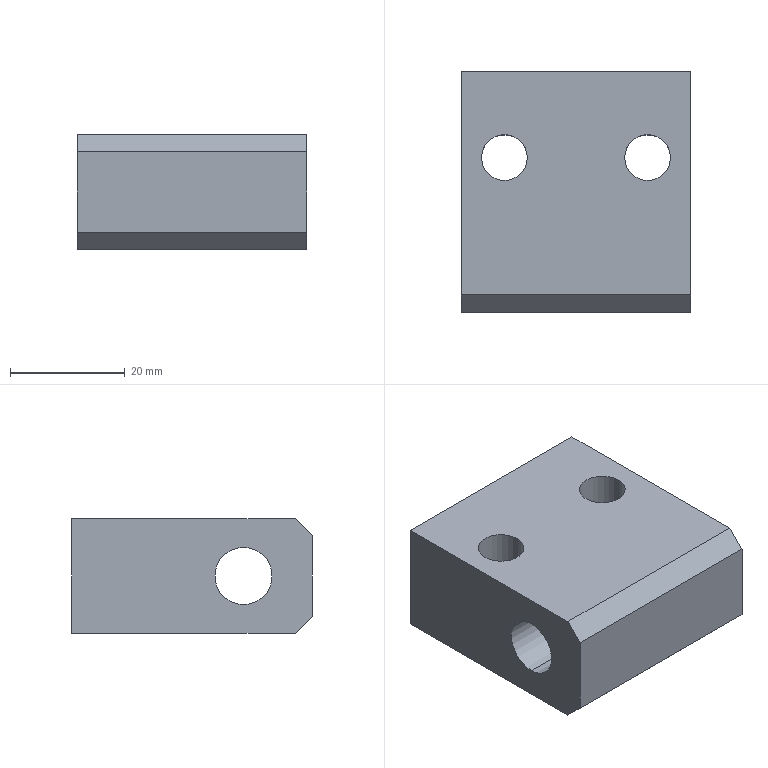Part | STEP file | HXGR200008-05-09 | 1 solid | 14 faces | box 40 x 42 x 20 mm | volume 28088 mm3 | plane 8 | cylinder 6 | commonest cylinder face diameters 8 x4 10 x2
STEP:
#1=CARTESIAN_POINT('',(-20.,-9.,5.));
#2=VERTEX_POINT('',#1);
#3=CARTESIAN_POINT('',(-20.,-9.,-5.));
#4=VERTEX_POINT('',#3);
#5=CARTESIAN_POINT('',(-20.,-9.,0.));
#6=DIRECTION('',(1.,0.,0.));
#7=DIRECTION('',(0.,0.,-1.));
#8=AXIS2_PLACEMENT_3D('',#5,#6,#7);
#9=CIRCLE('',#8,5.);
#10=EDGE_CURVE('',#2,#4,#9,.T.);
#11=ORIENTED_EDGE('',*,*,#10,.F.);
#12=CARTESIAN_POINT('',(20.,-9.,5.));
#13=VERTEX_POINT('',#12);
#14=CARTESIAN_POINT('',(20.,-9.,5.));
#15=DIRECTION('',(1.,0.,0.));
#16=VECTOR('',#15,1000.);
#17=LINE('',#14,#16);
#18=EDGE_CURVE('',#2,#13,#17,.T.);
#19=ORIENTED_EDGE('',*,*,#18,.T.);
#20=CARTESIAN_POINT('',(20.,-9.,-5.));
#21=VERTEX_POINT('',#20);
#22=CARTESIAN_POINT('',(20.,-9.,0.));
#23=DIRECTION('',(1.,0.,0.));
#24=DIRECTION('',(0.,0.,-1.));
#25=AXIS2_PLACEMENT_3D('',#22,#23,#24);
#26=CIRCLE('',#25,5.);
#27=EDGE_CURVE('',#13,#21,#26,.T.);
#28=ORIENTED_EDGE('',*,*,#27,.T.);
#29=CARTESIAN_POINT('',(20.,-9.,-5.));
#30=DIRECTION('',(1.,0.,0.));
#31=VECTOR('',#30,1000.);
#32=LINE('',#29,#31);
#33=EDGE_CURVE('',#4,#21,#32,.T.);
#34=ORIENTED_EDGE('',*,*,#33,.F.);
#35=EDGE_LOOP('',(#11,#19,#28,#34));
#36=FACE_OUTER_BOUND('',#35,.T.);
#37=CARTESIAN_POINT('',(20.,-9.,0.));
#38=DIRECTION('',(1.,0.,0.));
#39=DIRECTION('',(0.,0.,-1.));
#40=AXIS2_PLACEMENT_3D('',#37,#38,#39);
#41=CYLINDRICAL_SURFACE('',#40,5.);
#42=ADVANCED_FACE('',(#36),#41,.F.);
#43=CARTESIAN_POINT('',(-16.5,6.,-10.));
#44=VERTEX_POINT('',#43);
#45=CARTESIAN_POINT('',(-8.5,6.,-10.));
#46=VERTEX_POINT('',#45);
#47=CARTESIAN_POINT('',(-12.5,6.,-10.));
#48=DIRECTION('',(0.,0.,1.));
#49=DIRECTION('',(1.,0.,0.));
#50=AXIS2_PLACEMENT_3D('',#47,#48,#49);
#51=CIRCLE('',#50,4.);
#52=EDGE_CURVE('',#44,#46,#51,.T.);
#53=ORIENTED_EDGE('',*,*,#52,.F.);
#54=CARTESIAN_POINT('',(-16.5,6.,10.));
#55=VERTEX_POINT('',#54);
#56=CARTESIAN_POINT('',(-16.5,6.,10.));
#57=DIRECTION('',(0.,0.,1.));
#58=VECTOR('',#57,1000.);
#59=LINE('',#56,#58);
#60=EDGE_CURVE('',#44,#55,#59,.T.);
#61=ORIENTED_EDGE('',*,*,#60,.T.);
#62=CARTESIAN_POINT('',(-8.5,6.,10.));
#63=VERTEX_POINT('',#62);
#64=CARTESIAN_POINT('',(-12.5,6.,10.));
#65=DIRECTION('',(0.,0.,1.));
#66=DIRECTION('',(1.,0.,0.));
#67=AXIS2_PLACEMENT_3D('',#64,#65,#66);
#68=CIRCLE('',#67,4.);
#69=EDGE_CURVE('',#55,#63,#68,.T.);
#70=ORIENTED_EDGE('',*,*,#69,.T.);
#71=CARTESIAN_POINT('',(-8.5,6.,10.));
#72=DIRECTION('',(0.,0.,1.));
#73=VECTOR('',#72,1000.);
#74=LINE('',#71,#73);
#75=EDGE_CURVE('',#46,#63,#74,.T.);
#76=ORIENTED_EDGE('',*,*,#75,.F.);
#77=EDGE_LOOP('',(#53,#61,#70,#76));
#78=FACE_OUTER_BOUND('',#77,.T.);
#79=CARTESIAN_POINT('',(-12.5,6.,10.));
#80=DIRECTION('',(0.,0.,1.));
#81=DIRECTION('',(1.,0.,0.));
#82=AXIS2_PLACEMENT_3D('',#79,#80,#81);
#83=CYLINDRICAL_SURFACE('',#82,4.);
#84=ADVANCED_FACE('',(#78),#83,.F.);
#85=CARTESIAN_POINT('',(8.5,6.,-10.));
#86=VERTEX_POINT('',#85);
#87=CARTESIAN_POINT('',(16.5,6.,-10.));
#88=VERTEX_POINT('',#87);
#89=CARTESIAN_POINT('',(12.5,6.,-10.));
#90=DIRECTION('',(0.,0.,1.));
#91=DIRECTION('',(1.,0.,0.));
#92=AXIS2_PLACEMENT_3D('',#89,#90,#91);
#93=CIRCLE('',#92,4.);
#94=EDGE_CURVE('',#86,#88,#93,.T.);
#95=ORIENTED_EDGE('',*,*,#94,.F.);
#96=CARTESIAN_POINT('',(8.5,6.,10.));
#97=VERTEX_POINT('',#96);
#98=CARTESIAN_POINT('',(8.5,6.,10.));
#99=DIRECTION('',(0.,0.,1.));
#100=VECTOR('',#99,1000.);
#101=LINE('',#98,#100);
#102=EDGE_CURVE('',#86,#97,#101,.T.);
#103=ORIENTED_EDGE('',*,*,#102,.T.);
#104=CARTESIAN_POINT('',(16.5,6.,10.));
#105=VERTEX_POINT('',#104);
#106=CARTESIAN_POINT('',(12.5,6.,10.));
#107=DIRECTION('',(0.,0.,1.));
#108=DIRECTION('',(1.,0.,0.));
#109=AXIS2_PLACEMENT_3D('',#106,#107,#108);
#110=CIRCLE('',#109,4.);
#111=EDGE_CURVE('',#97,#105,#110,.T.);
#112=ORIENTED_EDGE('',*,*,#111,.T.);
#113=CARTESIAN_POINT('',(16.5,6.,10.));
#114=DIRECTION('',(0.,0.,1.));
#115=VECTOR('',#114,1000.);
#116=LINE('',#113,#115);
#117=EDGE_CURVE('',#88,#105,#116,.T.);
#118=ORIENTED_EDGE('',*,*,#117,.F.);
#119=EDGE_LOOP('',(#95,#103,#112,#118));
#120=FACE_OUTER_BOUND('',#119,.T.);
#121=CARTESIAN_POINT('',(12.5,6.,10.));
#122=DIRECTION('',(0.,0.,1.));
#123=DIRECTION('',(1.,0.,0.));
#124=AXIS2_PLACEMENT_3D('',#121,#122,#123);
#125=CYLINDRICAL_SURFACE('',#124,4.);
#126=ADVANCED_FACE('',(#120),#125,.F.);
#127=CARTESIAN_POINT('',(-20.,-9.,0.));
#128=DIRECTION('',(1.,0.,0.));
#129=DIRECTION('',(0.,0.,-1.));
#130=AXIS2_PLACEMENT_3D('',#127,#128,#129);
#131=CIRCLE('',#130,5.);
#132=EDGE_CURVE('',#4,#2,#131,.T.);
#133=ORIENTED_EDGE('',*,*,#132,.T.);
#134=ORIENTED_EDGE('',*,*,#10,.T.);
#135=EDGE_LOOP('',(#133,#134));
#136=FACE_BOUND('',#135,.T.);
#137=CARTESIAN_POINT('',(-20.,21.,-10.));
#138=VERTEX_POINT('',#137);
#139=CARTESIAN_POINT('',(-20.,-18.,-10.));
#140=VERTEX_POINT('',#139);
#141=CARTESIAN_POINT('',(-20.,-21.,-10.));
#142=DIRECTION('',(0.,-1.,0.));
#143=VECTOR('',#142,1000.);
#144=LINE('',#141,#143);
#145=EDGE_CURVE('',#138,#140,#144,.T.);
#146=ORIENTED_EDGE('',*,*,#145,.T.);
#147=CARTESIAN_POINT('',(-20.,-21.,-7.));
#148=VERTEX_POINT('',#147);
#149=CARTESIAN_POINT('',(-20.,-21.,-7.));
#150=DIRECTION('',(0.,-0.7071,0.7071));
#151=VECTOR('',#150,1000.);
#152=LINE('',#149,#151);
#153=EDGE_CURVE('',#140,#148,#152,.T.);
#154=ORIENTED_EDGE('',*,*,#153,.T.);
#155=CARTESIAN_POINT('',(-20.,-21.,7.));
#156=VERTEX_POINT('',#155);
#157=CARTESIAN_POINT('',(-20.,-21.,10.));
#158=DIRECTION('',(0.,0.,-1.));
#159=VECTOR('',#158,1000.);
#160=LINE('',#157,#159);
#161=EDGE_CURVE('',#156,#148,#160,.T.);
#162=ORIENTED_EDGE('',*,*,#161,.F.);
#163=CARTESIAN_POINT('',(-20.,-18.,10.));
#164=VERTEX_POINT('',#163);
#165=CARTESIAN_POINT('',(-20.,-18.,10.));
#166=DIRECTION('',(0.,0.7071,0.7071));
#167=VECTOR('',#166,1000.);
#168=LINE('',#165,#167);
#169=EDGE_CURVE('',#156,#164,#168,.T.);
#170=ORIENTED_EDGE('',*,*,#169,.T.);
#171=CARTESIAN_POINT('',(-20.,21.,10.));
#172=VERTEX_POINT('',#171);
#173=CARTESIAN_POINT('',(-20.,-21.,10.));
#174=DIRECTION('',(0.,-1.,0.));
#175=VECTOR('',#174,1000.);
#176=LINE('',#173,#175);
#177=EDGE_CURVE('',#172,#164,#176,.T.);
#178=ORIENTED_EDGE('',*,*,#177,.F.);
#179=CARTESIAN_POINT('',(-20.,21.,10.));
#180=DIRECTION('',(0.,0.,-1.));
#181=VECTOR('',#180,1000.);
#182=LINE('',#179,#181);
#183=EDGE_CURVE('',#172,#138,#182,.T.);
#184=ORIENTED_EDGE('',*,*,#183,.T.);
#185=EDGE_LOOP('',(#146,#154,#162,#170,#178,#184));
#186=FACE_OUTER_BOUND('',#185,.T.);
#187=CARTESIAN_POINT('',(-20.,-21.,10.));
#188=DIRECTION('',(1.,0.,0.));
#189=DIRECTION('',(0.,1.,0.));
#190=AXIS2_PLACEMENT_3D('',#187,#188,#189);
#191=PLANE('',#190);
#192=ADVANCED_FACE('',(#136,#186),#191,.F.);
#193=ORIENTED_EDGE('',*,*,#161,.T.);
#194=CARTESIAN_POINT('',(20.,-21.,-7.));
#195=VERTEX_POINT('',#194);
#196=CARTESIAN_POINT('',(20.,-21.,-7.));
#197=DIRECTION('',(1.,0.,0.));
#198=VECTOR('',#197,1000.);
#199=LINE('',#196,#198);
#200=EDGE_CURVE('',#148,#195,#199,.T.);
#201=ORIENTED_EDGE('',*,*,#200,.T.);
#202=CARTESIAN_POINT('',(20.,-21.,7.));
#203=VERTEX_POINT('',#202);
#204=CARTESIAN_POINT('',(20.,-21.,10.));
#205=DIRECTION('',(0.,0.,-1.));
#206=VECTOR('',#205,1000.);
#207=LINE('',#204,#206);
#208=EDGE_CURVE('',#203,#195,#207,.T.);
#209=ORIENTED_EDGE('',*,*,#208,.F.);
#210=CARTESIAN_POINT('',(-20.,-21.,7.));
#211=DIRECTION('',(-1.,0.,0.));
#212=VECTOR('',#211,1000.);
#213=LINE('',#210,#212);
#214=EDGE_CURVE('',#203,#156,#213,.T.);
#215=ORIENTED_EDGE('',*,*,#214,.T.);
#216=EDGE_LOOP('',(#193,#201,#209,#215));
#217=FACE_OUTER_BOUND('',#216,.T.);
#218=CARTESIAN_POINT('',(20.,-21.,10.));
#219=DIRECTION('',(0.,1.,0.));
#220=DIRECTION('',(-1.,0.,0.));
#221=AXIS2_PLACEMENT_3D('',#218,#219,#220);
#222=PLANE('',#221);
#223=ADVANCED_FACE('',(#217),#222,.F.);
#224=CARTESIAN_POINT('',(20.,-9.,0.));
#225=DIRECTION('',(1.,0.,0.));
#226=DIRECTION('',(0.,0.,-1.));
#227=AXIS2_PLACEMENT_3D('',#224,#225,#226);
#228=CIRCLE('',#227,5.);
#229=EDGE_CURVE('',#21,#13,#228,.T.);
#230=ORIENTED_EDGE('',*,*,#229,.F.);
#231=ORIENTED_EDGE('',*,*,#27,.F.);
#232=EDGE_LOOP('',(#230,#231));
#233=FACE_BOUND('',#232,.T.);
#234=ORIENTED_EDGE('',*,*,#208,.T.);
#235=CARTESIAN_POINT('',(20.,-18.,-10.));
#236=VERTEX_POINT('',#235);
#237=CARTESIAN_POINT('',(20.,-21.,-7.));
#238=DIRECTION('',(0.,0.7071,-0.7071));
#239=VECTOR('',#238,1000.);
#240=LINE('',#237,#239);
#241=EDGE_CURVE('',#195,#236,#240,.T.);
#242=ORIENTED_EDGE('',*,*,#241,.T.);
#243=CARTESIAN_POINT('',(20.,21.,-10.));
#244=VERTEX_POINT('',#243);
#245=CARTESIAN_POINT('',(20.,-21.,-10.));
#246=DIRECTION('',(0.,1.,0.));
#247=VECTOR('',#246,1000.);
#248=LINE('',#245,#247);
#249=EDGE_CURVE('',#236,#244,#248,.T.);
#250=ORIENTED_EDGE('',*,*,#249,.T.);
#251=CARTESIAN_POINT('',(20.,21.,10.));
#252=VERTEX_POINT('',#251);
#253=CARTESIAN_POINT('',(20.,21.,10.));
#254=DIRECTION('',(0.,0.,-1.));
#255=VECTOR('',#254,1000.);
#256=LINE('',#253,#255);
#257=EDGE_CURVE('',#252,#244,#256,.T.);
#258=ORIENTED_EDGE('',*,*,#257,.F.);
#259=CARTESIAN_POINT('',(20.,-18.,10.));
#260=VERTEX_POINT('',#259);
#261=CARTESIAN_POINT('',(20.,-21.,10.));
#262=DIRECTION('',(0.,1.,0.));
#263=VECTOR('',#262,1000.);
#264=LINE('',#261,#263);
#265=EDGE_CURVE('',#260,#252,#264,.T.);
#266=ORIENTED_EDGE('',*,*,#265,.F.);
#267=CARTESIAN_POINT('',(20.,-18.,10.));
#268=DIRECTION('',(0.,-0.7071,-0.7071));
#269=VECTOR('',#268,1000.);
#270=LINE('',#267,#269);
#271=EDGE_CURVE('',#260,#203,#270,.T.);
#272=ORIENTED_EDGE('',*,*,#271,.T.);
#273=EDGE_LOOP('',(#234,#242,#250,#258,#266,#272));
#274=FACE_OUTER_BOUND('',#273,.T.);
#275=CARTESIAN_POINT('',(20.,-21.,10.));
#276=DIRECTION('',(-1.,0.,0.));
#277=DIRECTION('',(0.,0.,1.));
#278=AXIS2_PLACEMENT_3D('',#275,#276,#277);
#279=PLANE('',#278);
#280=ADVANCED_FACE('',(#233,#274),#279,.F.);
#281=CARTESIAN_POINT('',(20.,21.,-10.));
#282=DIRECTION('',(-1.,0.,0.));
#283=VECTOR('',#282,1000.);
#284=LINE('',#281,#283);
#285=EDGE_CURVE('',#244,#138,#284,.T.);
#286=ORIENTED_EDGE('',*,*,#285,.T.);
#287=ORIENTED_EDGE('',*,*,#183,.F.);
#288=CARTESIAN_POINT('',(20.,21.,10.));
#289=DIRECTION('',(-1.,0.,0.));
#290=VECTOR('',#289,1000.);
#291=LINE('',#288,#290);
#292=EDGE_CURVE('',#252,#172,#291,.T.);
#293=ORIENTED_EDGE('',*,*,#292,.F.);
#294=ORIENTED_EDGE('',*,*,#257,.T.);
#295=EDGE_LOOP('',(#286,#287,#293,#294));
#296=FACE_OUTER_BOUND('',#295,.T.);
#297=CARTESIAN_POINT('',(20.,21.,10.));
#298=DIRECTION('',(0.,-1.,0.));
#299=DIRECTION('',(1.,0.,0.));
#300=AXIS2_PLACEMENT_3D('',#297,#298,#299);
#301=PLANE('',#300);
#302=ADVANCED_FACE('',(#296),#301,.F.);
#303=CARTESIAN_POINT('',(-12.5,6.,10.));
#304=DIRECTION('',(0.,0.,1.));
#305=DIRECTION('',(1.,0.,0.));
#306=AXIS2_PLACEMENT_3D('',#303,#304,#305);
#307=CIRCLE('',#306,4.);
#308=EDGE_CURVE('',#63,#55,#307,.T.);
#309=ORIENTED_EDGE('',*,*,#308,.F.);
#310=ORIENTED_EDGE('',*,*,#69,.F.);
#311=EDGE_LOOP('',(#309,#310));
#312=FACE_BOUND('',#311,.T.);
#313=CARTESIAN_POINT('',(12.5,6.,10.));
#314=DIRECTION('',(0.,0.,1.));
#315=DIRECTION('',(1.,0.,0.));
#316=AXIS2_PLACEMENT_3D('',#313,#314,#315);
#317=CIRCLE('',#316,4.);
#318=EDGE_CURVE('',#105,#97,#317,.T.);
#319=ORIENTED_EDGE('',*,*,#318,.F.);
#320=ORIENTED_EDGE('',*,*,#111,.F.);
#321=EDGE_LOOP('',(#319,#320));
#322=FACE_BOUND('',#321,.T.);
#323=ORIENTED_EDGE('',*,*,#177,.T.);
#324=CARTESIAN_POINT('',(20.,-18.,10.));
#325=DIRECTION('',(1.,0.,0.));
#326=VECTOR('',#325,1000.);
#327=LINE('',#324,#326);
#328=EDGE_CURVE('',#164,#260,#327,.T.);
#329=ORIENTED_EDGE('',*,*,#328,.T.);
#330=ORIENTED_EDGE('',*,*,#265,.T.);
#331=ORIENTED_EDGE('',*,*,#292,.T.);
#332=EDGE_LOOP('',(#323,#329,#330,#331));
#333=FACE_OUTER_BOUND('',#332,.T.);
#334=CARTESIAN_POINT('',(0.,0.,10.));
#335=DIRECTION('',(0.,0.,1.));
#336=DIRECTION('',(1.,0.,0.));
#337=AXIS2_PLACEMENT_3D('',#334,#335,#336);
#338=PLANE('',#337);
#339=ADVANCED_FACE('',(#312,#322,#333),#338,.T.);
#340=CARTESIAN_POINT('',(-12.5,6.,-10.));
#341=DIRECTION('',(0.,0.,1.));
#342=DIRECTION('',(1.,0.,0.));
#343=AXIS2_PLACEMENT_3D('',#340,#341,#342);
#344=CIRCLE('',#343,4.);
#345=EDGE_CURVE('',#46,#44,#344,.T.);
#346=ORIENTED_EDGE('',*,*,#345,.T.);
#347=ORIENTED_EDGE('',*,*,#52,.T.);
#348=EDGE_LOOP('',(#346,#347));
#349=FACE_BOUND('',#348,.T.);
#350=CARTESIAN_POINT('',(12.5,6.,-10.));
#351=DIRECTION('',(0.,0.,1.));
#352=DIRECTION('',(1.,0.,0.));
#353=AXIS2_PLACEMENT_3D('',#350,#351,#352);
#354=CIRCLE('',#353,4.);
#355=EDGE_CURVE('',#88,#86,#354,.T.);
#356=ORIENTED_EDGE('',*,*,#355,.T.);
#357=ORIENTED_EDGE('',*,*,#94,.T.);
#358=EDGE_LOOP('',(#356,#357));
#359=FACE_BOUND('',#358,.T.);
#360=ORIENTED_EDGE('',*,*,#249,.F.);
#361=CARTESIAN_POINT('',(0.,-18.,-10.));
#362=DIRECTION('',(-1.,0.,0.));
#363=VECTOR('',#362,1000.);
#364=LINE('',#361,#363);
#365=EDGE_CURVE('',#236,#140,#364,.T.);
#366=ORIENTED_EDGE('',*,*,#365,.T.);
#367=ORIENTED_EDGE('',*,*,#145,.F.);
#368=ORIENTED_EDGE('',*,*,#285,.F.);
#369=EDGE_LOOP('',(#360,#366,#367,#368));
#370=FACE_OUTER_BOUND('',#369,.T.);
#371=CARTESIAN_POINT('',(0.,0.,-10.));
#372=DIRECTION('',(0.,0.,1.));
#373=DIRECTION('',(1.,0.,0.));
#374=AXIS2_PLACEMENT_3D('',#371,#372,#373);
#375=PLANE('',#374);
#376=ADVANCED_FACE('',(#349,#359,#370),#375,.F.);
#377=ORIENTED_EDGE('',*,*,#102,.F.);
#378=ORIENTED_EDGE('',*,*,#355,.F.);
#379=ORIENTED_EDGE('',*,*,#117,.T.);
#380=ORIENTED_EDGE('',*,*,#318,.T.);
#381=EDGE_LOOP('',(#377,#378,#379,#380));
#382=FACE_OUTER_BOUND('',#381,.T.);
#383=CARTESIAN_POINT('',(12.5,6.,10.));
#384=DIRECTION('',(0.,0.,1.));
#385=DIRECTION('',(1.,0.,0.));
#386=AXIS2_PLACEMENT_3D('',#383,#384,#385);
#387=CYLINDRICAL_SURFACE('',#386,4.);
#388=ADVANCED_FACE('',(#382),#387,.F.);
#389=ORIENTED_EDGE('',*,*,#60,.F.);
#390=ORIENTED_EDGE('',*,*,#345,.F.);
#391=ORIENTED_EDGE('',*,*,#75,.T.);
#392=ORIENTED_EDGE('',*,*,#308,.T.);
#393=EDGE_LOOP('',(#389,#390,#391,#392));
#394=FACE_OUTER_BOUND('',#393,.T.);
#395=CARTESIAN_POINT('',(-12.5,6.,10.));
#396=DIRECTION('',(0.,0.,1.));
#397=DIRECTION('',(1.,0.,0.));
#398=AXIS2_PLACEMENT_3D('',#395,#396,#397);
#399=CYLINDRICAL_SURFACE('',#398,4.);
#400=ADVANCED_FACE('',(#394),#399,.F.);
#401=ORIENTED_EDGE('',*,*,#18,.F.);
#402=ORIENTED_EDGE('',*,*,#132,.F.);
#403=ORIENTED_EDGE('',*,*,#33,.T.);
#404=ORIENTED_EDGE('',*,*,#229,.T.);
#405=EDGE_LOOP('',(#401,#402,#403,#404));
#406=FACE_OUTER_BOUND('',#405,.T.);
#407=CARTESIAN_POINT('',(20.,-9.,0.));
#408=DIRECTION('',(1.,0.,0.));
#409=DIRECTION('',(0.,0.,-1.));
#410=AXIS2_PLACEMENT_3D('',#407,#408,#409);
#411=CYLINDRICAL_SURFACE('',#410,5.);
#412=ADVANCED_FACE('',(#406),#411,.F.);
#413=ORIENTED_EDGE('',*,*,#153,.F.);
#414=ORIENTED_EDGE('',*,*,#365,.F.);
#415=ORIENTED_EDGE('',*,*,#241,.F.);
#416=ORIENTED_EDGE('',*,*,#200,.F.);
#417=EDGE_LOOP('',(#413,#414,#415,#416));
#418=FACE_OUTER_BOUND('',#417,.T.);
#419=CARTESIAN_POINT('',(20.,-21.,-7.));
#420=DIRECTION('',(0.,0.7071,0.7071));
#421=DIRECTION('',(1.,0.,0.));
#422=AXIS2_PLACEMENT_3D('',#419,#420,#421);
#423=PLANE('',#422);
#424=ADVANCED_FACE('',(#418),#423,.F.);
#425=ORIENTED_EDGE('',*,*,#169,.F.);
#426=ORIENTED_EDGE('',*,*,#214,.F.);
#427=ORIENTED_EDGE('',*,*,#271,.F.);
#428=ORIENTED_EDGE('',*,*,#328,.F.);
#429=EDGE_LOOP('',(#425,#426,#427,#428));
#430=FACE_OUTER_BOUND('',#429,.T.);
#431=CARTESIAN_POINT('',(0.,-18.,10.));
#432=DIRECTION('',(0.,-0.7071,0.7071));
#433=DIRECTION('',(-1.,0.,0.));
#434=AXIS2_PLACEMENT_3D('',#431,#432,#433);
#435=PLANE('',#434);
#436=ADVANCED_FACE('',(#430),#435,.T.);
#437=CLOSED_SHELL('',(#42,#84,#126,#192,#223,#280,#302,#339,#376,#388,#400,#412,#424,#436));
#438=MANIFOLD_SOLID_BREP('',#437);
#439=CARTESIAN_POINT('',(0.,0.,0.));
#440=DIRECTION('',(0.,0.,1.));
#441=DIRECTION('',(1.,0.,0.));
#442=AXIS2_PLACEMENT_3D('',#439,#440,#441);
#443=(LENGTH_UNIT()NAMED_UNIT(*)SI_UNIT(.MILLI.,.METRE.));
#444=UNCERTAINTY_MEASURE_WITH_UNIT(LENGTH_MEASURE(0.00001),#443,'','');
#445=(NAMED_UNIT(*)PLANE_ANGLE_UNIT()SI_UNIT($,.RADIAN.));
#446=(NAMED_UNIT(*)SI_UNIT($,.STERADIAN.)SOLID_ANGLE_UNIT());
#447=(GEOMETRIC_REPRESENTATION_CONTEXT(3)GLOBAL_UNCERTAINTY_ASSIGNED_CONTEXT((#444))GLOBAL_UNIT_ASSIGNED_CONTEXT((#443,#445,#446))REPRESENTATION_CONTEXT('',''));
#448=ADVANCED_BREP_SHAPE_REPRESENTATION('',(#438,#442),#447);